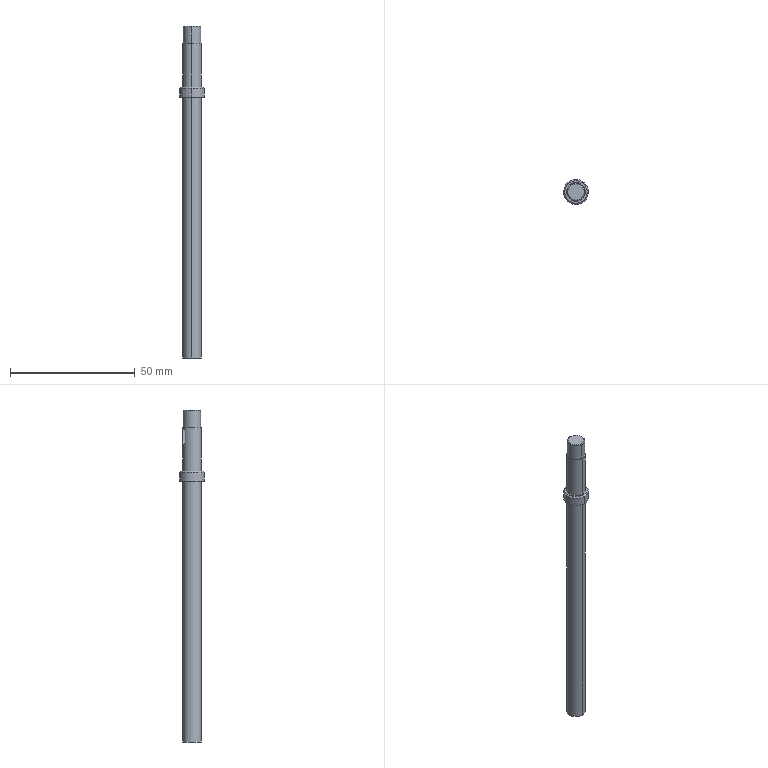Part | STEP file | 2026.6.15-Main Assembly图.sldasm-Part-112 | 1 solid | 22 faces | box 10 x 10 x 132.905 mm | volume 5947 mm3 | cylinder 10 | plane 8 | cone 4 | commonest cylinder face diameters 7.5 x4 2.5 x2 7 x2 10 x2
STEP:
#1=CARTESIAN_POINT('',(-1571.242,1419.764,3633.547));
#2=VERTEX_POINT('',#1);
#3=CARTESIAN_POINT('',(-1571.235,1428.764,3633.547));
#4=VERTEX_POINT('',#3);
#5=CARTESIAN_POINT('',(-1571.238,1424.264,3633.547));
#6=DIRECTION('',(0.,0.,1.));
#7=DIRECTION('',(-0.0007664,-1.,0.));
#8=AXIS2_PLACEMENT_3D('',#5,#6,#7);
#9=CIRCLE('',#8,4.5);
#10=EDGE_CURVE('',#2,#4,#9,.T.);
#11=ORIENTED_EDGE('',*,*,#10,.F.);
#12=CARTESIAN_POINT('',(-1571.242,1419.264,3633.047));
#13=VERTEX_POINT('',#12);
#14=CARTESIAN_POINT('',(-1571.242,1419.264,3633.047));
#15=DIRECTION('',(-0.000542,-0.7071,-0.7071));
#16=VECTOR('',#15,1000.);
#17=LINE('',#14,#16);
#18=EDGE_CURVE('',#2,#13,#17,.T.);
#19=ORIENTED_EDGE('',*,*,#18,.T.);
#20=CARTESIAN_POINT('',(-1571.044,1429.261,3633.047));
#21=VERTEX_POINT('',#20);
#22=CARTESIAN_POINT('',(-1571.238,1424.264,3633.047));
#23=DIRECTION('',(0.,0.,-1.));
#24=DIRECTION('',(-0.0007664,-1.,0.));
#25=AXIS2_PLACEMENT_3D('',#22,#23,#24);
#26=CIRCLE('',#25,5.);
#27=EDGE_CURVE('',#21,#13,#26,.T.);
#28=ORIENTED_EDGE('',*,*,#27,.F.);
#29=CARTESIAN_POINT('',(-1571.234,1429.264,3633.047));
#30=VERTEX_POINT('',#29);
#31=CARTESIAN_POINT('',(-1571.238,1424.264,3633.047));
#32=DIRECTION('',(0.,0.,-1.));
#33=DIRECTION('',(-0.0007664,-1.,0.));
#34=AXIS2_PLACEMENT_3D('',#31,#32,#33);
#35=CIRCLE('',#34,5.);
#36=EDGE_CURVE('',#30,#21,#35,.T.);
#37=ORIENTED_EDGE('',*,*,#36,.F.);
#38=CARTESIAN_POINT('',(-1571.234,1429.264,3633.047));
#39=DIRECTION('',(0.000542,0.7071,-0.7071));
#40=VECTOR('',#39,1000.);
#41=LINE('',#38,#40);
#42=EDGE_CURVE('',#4,#30,#41,.T.);
#43=ORIENTED_EDGE('',*,*,#42,.F.);
#44=EDGE_LOOP('',(#11,#19,#28,#37,#43));
#45=FACE_OUTER_BOUND('',#44,.T.);
#46=CARTESIAN_POINT('',(-1571.238,1424.264,3633.047));
#47=DIRECTION('',(0.,0.,-1.));
#48=DIRECTION('',(0.0007664,1.,0.));
#49=AXIS2_PLACEMENT_3D('',#46,#47,#48);
#50=CONICAL_SURFACE('',#49,5.,0.7854);
#51=ADVANCED_FACE('',(#45),#50,.T.);
#52=CARTESIAN_POINT('',(-1571.241,1421.014,3658.047));
#53=VERTEX_POINT('',#52);
#54=CARTESIAN_POINT('',(-1571.236,1427.514,3658.047));
#55=VERTEX_POINT('',#54);
#56=CARTESIAN_POINT('',(-1571.238,1424.264,3658.047));
#57=DIRECTION('',(0.,0.,1.));
#58=DIRECTION('',(-0.0007664,-1.,0.));
#59=AXIS2_PLACEMENT_3D('',#56,#57,#58);
#60=CIRCLE('',#59,3.25);
#61=EDGE_CURVE('',#53,#55,#60,.T.);
#62=ORIENTED_EDGE('',*,*,#61,.F.);
#63=CARTESIAN_POINT('',(-1571.241,1420.764,3657.797));
#64=VERTEX_POINT('',#63);
#65=CARTESIAN_POINT('',(-1571.241,1420.764,3657.797));
#66=DIRECTION('',(-0.000542,-0.7071,-0.7071));
#67=VECTOR('',#66,1000.);
#68=LINE('',#65,#67);
#69=EDGE_CURVE('',#53,#64,#68,.T.);
#70=ORIENTED_EDGE('',*,*,#69,.T.);
#71=CARTESIAN_POINT('',(-1571.102,1427.762,3657.797));
#72=VERTEX_POINT('',#71);
#73=CARTESIAN_POINT('',(-1571.238,1424.264,3657.797));
#74=DIRECTION('',(0.,0.,-1.));
#75=DIRECTION('',(-0.0007664,-1.,0.));
#76=AXIS2_PLACEMENT_3D('',#73,#74,#75);
#77=CIRCLE('',#76,3.5);
#78=EDGE_CURVE('',#72,#64,#77,.T.);
#79=ORIENTED_EDGE('',*,*,#78,.F.);
#80=CARTESIAN_POINT('',(-1571.236,1427.764,3657.797));
#81=VERTEX_POINT('',#80);
#82=CARTESIAN_POINT('',(-1571.238,1424.264,3657.797));
#83=DIRECTION('',(0.,0.,-1.));
#84=DIRECTION('',(-0.0007664,-1.,0.));
#85=AXIS2_PLACEMENT_3D('',#82,#83,#84);
#86=CIRCLE('',#85,3.5);
#87=EDGE_CURVE('',#81,#72,#86,.T.);
#88=ORIENTED_EDGE('',*,*,#87,.F.);
#89=CARTESIAN_POINT('',(-1571.236,1427.764,3657.797));
#90=DIRECTION('',(0.000542,0.7071,-0.7071));
#91=VECTOR('',#90,1000.);
#92=LINE('',#89,#91);
#93=EDGE_CURVE('',#55,#81,#92,.T.);
#94=ORIENTED_EDGE('',*,*,#93,.F.);
#95=EDGE_LOOP('',(#62,#70,#79,#88,#94));
#96=FACE_OUTER_BOUND('',#95,.T.);
#97=CARTESIAN_POINT('',(-1571.238,1424.264,3657.797));
#98=DIRECTION('',(0.,0.,-1.));
#99=DIRECTION('',(0.0007664,1.,0.));
#100=AXIS2_PLACEMENT_3D('',#97,#98,#99);
#101=CONICAL_SURFACE('',#100,3.5,0.7854);
#102=ADVANCED_FACE('',(#96),#101,.T.);
#103=ORIENTED_EDGE('',*,*,#27,.T.);
#104=CARTESIAN_POINT('',(-1571.433,1419.268,3633.047));
#105=VERTEX_POINT('',#104);
#106=CARTESIAN_POINT('',(-1571.238,1424.264,3633.047));
#107=DIRECTION('',(0.,0.,-1.));
#108=DIRECTION('',(-0.0007664,-1.,0.));
#109=AXIS2_PLACEMENT_3D('',#106,#107,#108);
#110=CIRCLE('',#109,5.);
#111=EDGE_CURVE('',#13,#105,#110,.T.);
#112=ORIENTED_EDGE('',*,*,#111,.T.);
#113=CARTESIAN_POINT('',(-1571.433,1419.268,3629.547));
#114=VERTEX_POINT('',#113);
#115=CARTESIAN_POINT('',(-1571.433,1419.268,3633.547));
#116=DIRECTION('',(0.,0.,-1.));
#117=VECTOR('',#116,1000.);
#118=LINE('',#115,#117);
#119=EDGE_CURVE('',#105,#114,#118,.T.);
#120=ORIENTED_EDGE('',*,*,#119,.T.);
#121=CARTESIAN_POINT('',(-1571.044,1429.261,3629.547));
#122=VERTEX_POINT('',#121);
#123=CARTESIAN_POINT('',(-1571.238,1424.264,3629.547));
#124=DIRECTION('',(0.,0.,1.));
#125=DIRECTION('',(0.03892,0.9992,0.));
#126=AXIS2_PLACEMENT_3D('',#123,#124,#125);
#127=CIRCLE('',#126,5.);
#128=EDGE_CURVE('',#114,#122,#127,.T.);
#129=ORIENTED_EDGE('',*,*,#128,.T.);
#130=CARTESIAN_POINT('',(-1571.044,1429.261,3633.547));
#131=DIRECTION('',(0.,0.,-1.));
#132=VECTOR('',#131,1000.);
#133=LINE('',#130,#132);
#134=EDGE_CURVE('',#21,#122,#133,.T.);
#135=ORIENTED_EDGE('',*,*,#134,.F.);
#136=EDGE_LOOP('',(#103,#112,#120,#129,#135));
#137=FACE_OUTER_BOUND('',#136,.T.);
#138=CARTESIAN_POINT('',(-1571.238,1424.264,3633.547));
#139=DIRECTION('',(0.,0.,-1.));
#140=DIRECTION('',(0.03892,0.9992,0.));
#141=AXIS2_PLACEMENT_3D('',#138,#139,#140);
#142=CYLINDRICAL_SURFACE('',#141,5.);
#143=ADVANCED_FACE('',(#137),#142,.T.);
#144=CARTESIAN_POINT('',(-1571.092,1428.011,3651.047));
#145=VERTEX_POINT('',#144);
#146=CARTESIAN_POINT('',(-1571.384,1420.517,3651.047));
#147=VERTEX_POINT('',#146);
#148=CARTESIAN_POINT('',(-1571.238,1424.264,3651.047));
#149=DIRECTION('',(0.,0.,-1.));
#150=DIRECTION('',(0.03892,0.9992,0.));
#151=AXIS2_PLACEMENT_3D('',#148,#149,#150);
#152=CIRCLE('',#151,3.75);
#153=EDGE_CURVE('',#145,#147,#152,.T.);
#154=ORIENTED_EDGE('',*,*,#153,.T.);
#155=CARTESIAN_POINT('',(-1571.384,1420.517,3633.547));
#156=VERTEX_POINT('',#155);
#157=CARTESIAN_POINT('',(-1571.384,1420.517,3651.047));
#158=DIRECTION('',(0.,0.,-1.));
#159=VECTOR('',#158,1000.);
#160=LINE('',#157,#159);
#161=EDGE_CURVE('',#147,#156,#160,.T.);
#162=ORIENTED_EDGE('',*,*,#161,.T.);
#163=CARTESIAN_POINT('',(-1571.092,1428.011,3633.547));
#164=VERTEX_POINT('',#163);
#165=CARTESIAN_POINT('',(-1571.238,1424.264,3633.547));
#166=DIRECTION('',(0.,0.,1.));
#167=DIRECTION('',(0.03892,0.9992,0.));
#168=AXIS2_PLACEMENT_3D('',#165,#166,#167);
#169=CIRCLE('',#168,3.75);
#170=EDGE_CURVE('',#156,#164,#169,.T.);
#171=ORIENTED_EDGE('',*,*,#170,.T.);
#172=CARTESIAN_POINT('',(-1571.092,1428.011,3651.047));
#173=DIRECTION('',(0.,0.,-1.));
#174=VECTOR('',#173,1000.);
#175=LINE('',#172,#174);
#176=EDGE_CURVE('',#145,#164,#175,.T.);
#177=ORIENTED_EDGE('',*,*,#176,.F.);
#178=EDGE_LOOP('',(#154,#162,#171,#177));
#179=FACE_OUTER_BOUND('',#178,.T.);
#180=CARTESIAN_POINT('',(-1571.238,1424.264,3651.047));
#181=DIRECTION('',(0.,0.,-1.));
#182=DIRECTION('',(0.03892,0.9992,0.));
#183=AXIS2_PLACEMENT_3D('',#180,#181,#182);
#184=CYLINDRICAL_SURFACE('',#183,3.75);
#185=ADVANCED_FACE('',(#179),#184,.T.);
#186=ORIENTED_EDGE('',*,*,#78,.T.);
#187=CARTESIAN_POINT('',(-1571.374,1420.767,3657.797));
#188=VERTEX_POINT('',#187);
#189=CARTESIAN_POINT('',(-1571.238,1424.264,3657.797));
#190=DIRECTION('',(0.,0.,-1.));
#191=DIRECTION('',(-0.0007664,-1.,0.));
#192=AXIS2_PLACEMENT_3D('',#189,#190,#191);
#193=CIRCLE('',#192,3.5);
#194=EDGE_CURVE('',#64,#188,#193,.T.);
#195=ORIENTED_EDGE('',*,*,#194,.T.);
#196=CARTESIAN_POINT('',(-1571.374,1420.767,3651.047));
#197=VERTEX_POINT('',#196);
#198=CARTESIAN_POINT('',(-1571.374,1420.767,3658.047));
#199=DIRECTION('',(0.,0.,-1.));
#200=VECTOR('',#199,1000.);
#201=LINE('',#198,#200);
#202=EDGE_CURVE('',#188,#197,#201,.T.);
#203=ORIENTED_EDGE('',*,*,#202,.T.);
#204=CARTESIAN_POINT('',(-1571.102,1427.762,3651.047));
#205=VERTEX_POINT('',#204);
#206=CARTESIAN_POINT('',(-1571.238,1424.264,3651.047));
#207=DIRECTION('',(0.,0.,1.));
#208=DIRECTION('',(0.03892,0.9992,0.));
#209=AXIS2_PLACEMENT_3D('',#206,#207,#208);
#210=CIRCLE('',#209,3.5);
#211=EDGE_CURVE('',#197,#205,#210,.T.);
#212=ORIENTED_EDGE('',*,*,#211,.T.);
#213=CARTESIAN_POINT('',(-1571.102,1427.762,3658.047));
#214=DIRECTION('',(0.,0.,-1.));
#215=VECTOR('',#214,1000.);
#216=LINE('',#213,#215);
#217=EDGE_CURVE('',#72,#205,#216,.T.);
#218=ORIENTED_EDGE('',*,*,#217,.F.);
#219=EDGE_LOOP('',(#186,#195,#203,#212,#218));
#220=FACE_OUTER_BOUND('',#219,.T.);
#221=CARTESIAN_POINT('',(-1571.238,1424.264,3658.047));
#222=DIRECTION('',(0.,0.,-1.));
#223=DIRECTION('',(0.03892,0.9992,0.));
#224=AXIS2_PLACEMENT_3D('',#221,#222,#223);
#225=CYLINDRICAL_SURFACE('',#224,3.5);
#226=ADVANCED_FACE('',(#220),#225,.T.);
#227=CARTESIAN_POINT('',(-1571.092,1428.011,3629.547));
#228=VERTEX_POINT('',#227);
#229=CARTESIAN_POINT('',(-1571.384,1420.517,3629.547));
#230=VERTEX_POINT('',#229);
#231=CARTESIAN_POINT('',(-1571.238,1424.264,3629.547));
#232=DIRECTION('',(0.,0.,-1.));
#233=DIRECTION('',(0.03892,0.9992,0.));
#234=AXIS2_PLACEMENT_3D('',#231,#232,#233);
#235=CIRCLE('',#234,3.75);
#236=EDGE_CURVE('',#228,#230,#235,.T.);
#237=ORIENTED_EDGE('',*,*,#236,.T.);
#238=CARTESIAN_POINT('',(-1571.384,1420.517,3525.142));
#239=VERTEX_POINT('',#238);
#240=CARTESIAN_POINT('',(-1571.384,1420.517,3629.547));
#241=DIRECTION('',(0.,0.,-1.));
#242=VECTOR('',#241,1000.);
#243=LINE('',#240,#242);
#244=EDGE_CURVE('',#230,#239,#243,.T.);
#245=ORIENTED_EDGE('',*,*,#244,.T.);
#246=CARTESIAN_POINT('',(-1571.092,1428.011,3525.142));
#247=VERTEX_POINT('',#246);
#248=CARTESIAN_POINT('',(-1571.238,1424.264,3525.142));
#249=DIRECTION('',(0.,0.,-1.));
#250=DIRECTION('',(1.,0.,0.));
#251=AXIS2_PLACEMENT_3D('',#248,#249,#250);
#252=CIRCLE('',#251,3.75);
#253=EDGE_CURVE('',#247,#239,#252,.T.);
#254=ORIENTED_EDGE('',*,*,#253,.F.);
#255=CARTESIAN_POINT('',(-1571.092,1428.011,3629.547));
#256=DIRECTION('',(0.,0.,-1.));
#257=VECTOR('',#256,1000.);
#258=LINE('',#255,#257);
#259=EDGE_CURVE('',#228,#247,#258,.T.);
#260=ORIENTED_EDGE('',*,*,#259,.F.);
#261=EDGE_LOOP('',(#237,#245,#254,#260));
#262=FACE_OUTER_BOUND('',#261,.T.);
#263=CARTESIAN_POINT('',(-1571.238,1424.264,3629.547));
#264=DIRECTION('',(0.,0.,-1.));
#265=DIRECTION('',(0.03892,0.9992,0.));
#266=AXIS2_PLACEMENT_3D('',#263,#264,#265);
#267=CYLINDRICAL_SURFACE('',#266,3.75);
#268=ADVANCED_FACE('',(#262),#267,.T.);
#269=ORIENTED_EDGE('',*,*,#244,.F.);
#270=CARTESIAN_POINT('',(-1571.238,1424.264,3629.547));
#271=DIRECTION('',(0.,0.,-1.));
#272=DIRECTION('',(0.03892,0.9992,0.));
#273=AXIS2_PLACEMENT_3D('',#270,#271,#272);
#274=CIRCLE('',#273,3.75);
#275=EDGE_CURVE('',#230,#228,#274,.T.);
#276=ORIENTED_EDGE('',*,*,#275,.T.);
#277=ORIENTED_EDGE('',*,*,#259,.T.);
#278=CARTESIAN_POINT('',(-1571.238,1424.264,3525.142));
#279=DIRECTION('',(0.,0.,-1.));
#280=DIRECTION('',(1.,0.,0.));
#281=AXIS2_PLACEMENT_3D('',#278,#279,#280);
#282=CIRCLE('',#281,3.75);
#283=EDGE_CURVE('',#239,#247,#282,.T.);
#284=ORIENTED_EDGE('',*,*,#283,.F.);
#285=EDGE_LOOP('',(#269,#276,#277,#284));
#286=FACE_OUTER_BOUND('',#285,.T.);
#287=CARTESIAN_POINT('',(-1571.238,1424.264,3629.547));
#288=DIRECTION('',(0.,0.,-1.));
#289=DIRECTION('',(0.03892,0.9992,0.));
#290=AXIS2_PLACEMENT_3D('',#287,#288,#289);
#291=CYLINDRICAL_SURFACE('',#290,3.75);
#292=ADVANCED_FACE('',(#286),#291,.T.);
#293=CARTESIAN_POINT('',(-1571.238,1424.264,3658.047));
#294=DIRECTION('',(0.,0.,1.));
#295=DIRECTION('',(-0.0007664,-1.,0.));
#296=AXIS2_PLACEMENT_3D('',#293,#294,#295);
#297=CIRCLE('',#296,3.25);
#298=EDGE_CURVE('',#55,#53,#297,.T.);
#299=ORIENTED_EDGE('',*,*,#298,.T.);
#300=ORIENTED_EDGE('',*,*,#61,.T.);
#301=EDGE_LOOP('',(#299,#300));
#302=FACE_OUTER_BOUND('',#301,.T.);
#303=CARTESIAN_POINT('',(-1571.238,1424.264,3658.047));
#304=DIRECTION('',(0.,0.,1.));
#305=DIRECTION('',(-0.0007664,-1.,0.));
#306=AXIS2_PLACEMENT_3D('',#303,#304,#305);
#307=PLANE('',#306);
#308=ADVANCED_FACE('',(#302),#307,.T.);
#309=ORIENTED_EDGE('',*,*,#202,.F.);
#310=CARTESIAN_POINT('',(-1571.238,1424.264,3657.797));
#311=DIRECTION('',(0.,0.,-1.));
#312=DIRECTION('',(-0.0007664,-1.,0.));
#313=AXIS2_PLACEMENT_3D('',#310,#311,#312);
#314=CIRCLE('',#313,3.5);
#315=EDGE_CURVE('',#188,#81,#314,.T.);
#316=ORIENTED_EDGE('',*,*,#315,.T.);
#317=ORIENTED_EDGE('',*,*,#87,.T.);
#318=ORIENTED_EDGE('',*,*,#217,.T.);
#319=CARTESIAN_POINT('',(-1571.238,1424.264,3651.047));
#320=DIRECTION('',(0.,0.,1.));
#321=DIRECTION('',(0.03892,0.9992,0.));
#322=AXIS2_PLACEMENT_3D('',#319,#320,#321);
#323=CIRCLE('',#322,3.5);
#324=EDGE_CURVE('',#205,#197,#323,.T.);
#325=ORIENTED_EDGE('',*,*,#324,.T.);
#326=EDGE_LOOP('',(#309,#316,#317,#318,#325));
#327=FACE_OUTER_BOUND('',#326,.T.);
#328=CARTESIAN_POINT('',(-1571.238,1424.264,3658.047));
#329=DIRECTION('',(0.,0.,-1.));
#330=DIRECTION('',(0.03892,0.9992,0.));
#331=AXIS2_PLACEMENT_3D('',#328,#329,#330);
#332=CYLINDRICAL_SURFACE('',#331,3.5);
#333=ADVANCED_FACE('',(#327),#332,.T.);
#334=ORIENTED_EDGE('',*,*,#324,.F.);
#335=ORIENTED_EDGE('',*,*,#211,.F.);
#336=EDGE_LOOP('',(#334,#335));
#337=FACE_BOUND('',#336,.T.);
#338=ORIENTED_EDGE('',*,*,#153,.F.);
#339=CARTESIAN_POINT('',(-1571.238,1424.264,3651.047));
#340=DIRECTION('',(0.,0.,-1.));
#341=DIRECTION('',(0.03892,0.9992,0.));
#342=AXIS2_PLACEMENT_3D('',#339,#340,#341);
#343=CIRCLE('',#342,3.75);
#344=EDGE_CURVE('',#147,#145,#343,.T.);
#345=ORIENTED_EDGE('',*,*,#344,.F.);
#346=EDGE_LOOP('',(#338,#345));
#347=FACE_OUTER_BOUND('',#346,.T.);
#348=CARTESIAN_POINT('',(-1571.238,1424.264,3651.047));
#349=DIRECTION('',(0.,0.,1.));
#350=DIRECTION('',(-0.0007664,-1.,0.));
#351=AXIS2_PLACEMENT_3D('',#348,#349,#350);
#352=PLANE('',#351);
#353=ADVANCED_FACE('',(#337,#347),#352,.T.);
#354=ORIENTED_EDGE('',*,*,#161,.F.);
#355=ORIENTED_EDGE('',*,*,#344,.T.);
#356=ORIENTED_EDGE('',*,*,#176,.T.);
#357=CARTESIAN_POINT('',(-1571.238,1424.264,3633.547));
#358=DIRECTION('',(0.,0.,1.));
#359=DIRECTION('',(0.03892,0.9992,0.));
#360=AXIS2_PLACEMENT_3D('',#357,#358,#359);
#361=CIRCLE('',#360,3.75);
#362=EDGE_CURVE('',#164,#156,#361,.T.);
#363=ORIENTED_EDGE('',*,*,#362,.T.);
#364=EDGE_LOOP('',(#354,#355,#356,#363));
#365=FACE_OUTER_BOUND('',#364,.T.);
#366=CARTESIAN_POINT('',(-1571.607,1427.996,3645.547));
#367=VERTEX_POINT('',#366);
#368=CARTESIAN_POINT('',(-1573.871,1426.935,3645.547));
#369=VERTEX_POINT('',#368);
#370=CARTESIAN_POINT('',(-1571.607,1427.996,3645.547));
#371=CARTESIAN_POINT('',(-1571.607,1427.996,3645.38));
#372=CARTESIAN_POINT('',(-1571.642,1427.993,3645.217));
#373=CARTESIAN_POINT('',(-1571.773,1427.977,3644.915));
#374=CARTESIAN_POINT('',(-1571.869,1427.963,3644.777));
#375=CARTESIAN_POINT('',(-1572.1,1427.916,3644.549));
#376=CARTESIAN_POINT('',(-1572.237,1427.882,3644.456));
#377=CARTESIAN_POINT('',(-1572.525,1427.79,3644.331));
#378=CARTESIAN_POINT('',(-1572.68,1427.73,3644.297));
#379=CARTESIAN_POINT('',(-1572.903,1427.626,3644.297));
#380=CARTESIAN_POINT('',(-1572.977,1427.588,3644.305));
#381=CARTESIAN_POINT('',(-1573.119,1427.51,3644.337));
#382=CARTESIAN_POINT('',(-1573.186,1427.47,3644.361));
#383=CARTESIAN_POINT('',(-1573.38,1427.346,3644.456));
#384=CARTESIAN_POINT('',(-1573.493,1427.263,3644.548));
#385=CARTESIAN_POINT('',(-1573.631,1427.152,3644.72));
#386=CARTESIAN_POINT('',(-1573.672,1427.118,3644.783));
#387=CARTESIAN_POINT('',(-1573.743,1427.056,3644.918));
#388=CARTESIAN_POINT('',(-1573.773,1427.028,3644.991));
#389=CARTESIAN_POINT('',(-1573.845,1426.961,3645.216));
#390=CARTESIAN_POINT('',(-1573.871,1426.935,3645.38));
#391=CARTESIAN_POINT('',(-1573.871,1426.935,3645.547));
#392=B_SPLINE_CURVE_WITH_KNOTS('',3,(#370,#371,#372,#373,#374,#375,#376,#377,#378,#379,#380,#381,#382,#383,#384,#385,#386,#387,#388,#389,#390,#391),.UNSPECIFIED.,.F.,.F.,(4,2,2,2,2,2,2,2,2,2,4),(0.,0.0004919,0.0009837,0.001476,0.001967,0.002213,0.002459,0.002951,0.003197,0.003443,0.003935),.UNSPECIFIED.);
#393=EDGE_CURVE('',#367,#369,#392,.T.);
#394=ORIENTED_EDGE('',*,*,#393,.F.);
#395=CARTESIAN_POINT('',(-1571.607,1427.996,3649.547));
#396=VERTEX_POINT('',#395);
#397=CARTESIAN_POINT('',(-1571.607,1427.996,3651.047));
#398=DIRECTION('',(0.,0.,1.));
#399=VECTOR('',#398,1000.);
#400=LINE('',#397,#399);
#401=EDGE_CURVE('',#367,#396,#400,.T.);
#402=ORIENTED_EDGE('',*,*,#401,.T.);
#403=CARTESIAN_POINT('',(-1573.871,1426.935,3649.547));
#404=VERTEX_POINT('',#403);
#405=CARTESIAN_POINT('',(-1573.871,1426.935,3649.547));
#406=CARTESIAN_POINT('',(-1573.871,1426.935,3649.713));
#407=CARTESIAN_POINT('',(-1573.846,1426.96,3649.876));
#408=CARTESIAN_POINT('',(-1573.749,1427.05,3650.178));
#409=CARTESIAN_POINT('',(-1573.677,1427.115,3650.316));
#410=CARTESIAN_POINT('',(-1573.494,1427.263,3650.545));
#411=CARTESIAN_POINT('',(-1573.38,1427.346,3650.638));
#412=CARTESIAN_POINT('',(-1573.125,1427.509,3650.763));
#413=CARTESIAN_POINT('',(-1572.98,1427.589,3650.797));
#414=CARTESIAN_POINT('',(-1572.757,1427.694,3650.797));
#415=CARTESIAN_POINT('',(-1572.68,1427.727,3650.789));
#416=CARTESIAN_POINT('',(-1572.53,1427.786,3650.757));
#417=CARTESIAN_POINT('',(-1572.456,1427.812,3650.733));
#418=CARTESIAN_POINT('',(-1572.237,1427.882,3650.638));
#419=CARTESIAN_POINT('',(-1572.101,1427.916,3650.546));
#420=CARTESIAN_POINT('',(-1571.927,1427.951,3650.373));
#421=CARTESIAN_POINT('',(-1571.874,1427.96,3650.311));
#422=CARTESIAN_POINT('',(-1571.781,1427.975,3650.176));
#423=CARTESIAN_POINT('',(-1571.741,1427.981,3650.103));
#424=CARTESIAN_POINT('',(-1571.643,1427.993,3649.878));
#425=CARTESIAN_POINT('',(-1571.607,1427.996,3649.713));
#426=CARTESIAN_POINT('',(-1571.607,1427.996,3649.547));
#427=B_SPLINE_CURVE_WITH_KNOTS('',3,(#405,#406,#407,#408,#409,#410,#411,#412,#413,#414,#415,#416,#417,#418,#419,#420,#421,#422,#423,#424,#425,#426),.UNSPECIFIED.,.F.,.F.,(4,2,2,2,2,2,2,2,2,2,4),(0.,0.0004919,0.0009837,0.001476,0.001967,0.002213,0.002459,0.002951,0.003197,0.003443,0.003935),.UNSPECIFIED.);
#428=EDGE_CURVE('',#404,#396,#427,.T.);
#429=ORIENTED_EDGE('',*,*,#428,.F.);
#430=CARTESIAN_POINT('',(-1573.871,1426.935,3651.047));
#431=DIRECTION('',(0.,0.,-1.));
#432=VECTOR('',#431,1000.);
#433=LINE('',#430,#432);
#434=EDGE_CURVE('',#404,#369,#433,.T.);
#435=ORIENTED_EDGE('',*,*,#434,.T.);
#436=EDGE_LOOP('',(#394,#402,#429,#435));
#437=FACE_BOUND('',#436,.T.);
#438=CARTESIAN_POINT('',(-1571.238,1424.264,3651.047));
#439=DIRECTION('',(0.,0.,-1.));
#440=DIRECTION('',(0.03892,0.9992,0.));
#441=AXIS2_PLACEMENT_3D('',#438,#439,#440);
#442=CYLINDRICAL_SURFACE('',#441,3.75);
#443=ADVANCED_FACE('',(#365,#437),#442,.T.);
#444=ORIENTED_EDGE('',*,*,#236,.F.);
#445=ORIENTED_EDGE('',*,*,#275,.F.);
#446=EDGE_LOOP('',(#444,#445));
#447=FACE_BOUND('',#446,.T.);
#448=CARTESIAN_POINT('',(-1571.238,1424.264,3629.547));
#449=DIRECTION('',(0.,0.,1.));
#450=DIRECTION('',(0.03892,0.9992,0.));
#451=AXIS2_PLACEMENT_3D('',#448,#449,#450);
#452=CIRCLE('',#451,5.);
#453=EDGE_CURVE('',#122,#114,#452,.T.);
#454=ORIENTED_EDGE('',*,*,#453,.F.);
#455=ORIENTED_EDGE('',*,*,#128,.F.);
#456=EDGE_LOOP('',(#454,#455));
#457=FACE_OUTER_BOUND('',#456,.T.);
#458=CARTESIAN_POINT('',(-1571.238,1424.264,3629.547));
#459=DIRECTION('',(0.,0.,-1.));
#460=DIRECTION('',(0.0007664,1.,0.));
#461=AXIS2_PLACEMENT_3D('',#458,#459,#460);
#462=PLANE('',#461);
#463=ADVANCED_FACE('',(#447,#457),#462,.T.);
#464=CARTESIAN_POINT('',(-1571.238,1424.264,3633.547));
#465=DIRECTION('',(0.,0.,1.));
#466=DIRECTION('',(-0.0007664,-1.,0.));
#467=AXIS2_PLACEMENT_3D('',#464,#465,#466);
#468=CIRCLE('',#467,4.5);
#469=EDGE_CURVE('',#4,#2,#468,.T.);
#470=ORIENTED_EDGE('',*,*,#469,.T.);
#471=ORIENTED_EDGE('',*,*,#10,.T.);
#472=EDGE_LOOP('',(#470,#471));
#473=FACE_OUTER_BOUND('',#472,.T.);
#474=ORIENTED_EDGE('',*,*,#362,.F.);
#475=ORIENTED_EDGE('',*,*,#170,.F.);
#476=EDGE_LOOP('',(#474,#475));
#477=FACE_BOUND('',#476,.T.);
#478=CARTESIAN_POINT('',(-1571.238,1424.264,3633.547));
#479=DIRECTION('',(0.,0.,1.));
#480=DIRECTION('',(-0.0007664,-1.,0.));
#481=AXIS2_PLACEMENT_3D('',#478,#479,#480);
#482=PLANE('',#481);
#483=ADVANCED_FACE('',(#473,#477),#482,.T.);
#484=ORIENTED_EDGE('',*,*,#119,.F.);
#485=CARTESIAN_POINT('',(-1571.238,1424.264,3633.047));
#486=DIRECTION('',(0.,0.,-1.));
#487=DIRECTION('',(-0.0007664,-1.,0.));
#488=AXIS2_PLACEMENT_3D('',#485,#486,#487);
#489=CIRCLE('',#488,5.);
#490=EDGE_CURVE('',#105,#30,#489,.T.);
#491=ORIENTED_EDGE('',*,*,#490,.T.);
#492=ORIENTED_EDGE('',*,*,#36,.T.);
#493=ORIENTED_EDGE('',*,*,#134,.T.);
#494=ORIENTED_EDGE('',*,*,#453,.T.);
#495=EDGE_LOOP('',(#484,#491,#492,#493,#494));
#496=FACE_OUTER_BOUND('',#495,.T.);
#497=CARTESIAN_POINT('',(-1571.238,1424.264,3633.547));
#498=DIRECTION('',(0.,0.,-1.));
#499=DIRECTION('',(0.03892,0.9992,0.));
#500=AXIS2_PLACEMENT_3D('',#497,#498,#499);
#501=CYLINDRICAL_SURFACE('',#500,5.);
#502=ADVANCED_FACE('',(#496),#501,.T.);
#503=ORIENTED_EDGE('',*,*,#69,.F.);
#504=ORIENTED_EDGE('',*,*,#298,.F.);
#505=ORIENTED_EDGE('',*,*,#93,.T.);
#506=ORIENTED_EDGE('',*,*,#315,.F.);
#507=ORIENTED_EDGE('',*,*,#194,.F.);
#508=EDGE_LOOP('',(#503,#504,#505,#506,#507));
#509=FACE_OUTER_BOUND('',#508,.T.);
#510=CARTESIAN_POINT('',(-1571.238,1424.264,3657.797));
#511=DIRECTION('',(0.,0.,-1.));
#512=DIRECTION('',(0.0007664,1.,0.));
#513=AXIS2_PLACEMENT_3D('',#510,#511,#512);
#514=CONICAL_SURFACE('',#513,3.5,0.7854);
#515=ADVANCED_FACE('',(#509),#514,.T.);
#516=ORIENTED_EDGE('',*,*,#18,.F.);
#517=ORIENTED_EDGE('',*,*,#469,.F.);
#518=ORIENTED_EDGE('',*,*,#42,.T.);
#519=ORIENTED_EDGE('',*,*,#490,.F.);
#520=ORIENTED_EDGE('',*,*,#111,.F.);
#521=EDGE_LOOP('',(#516,#517,#518,#519,#520));
#522=FACE_OUTER_BOUND('',#521,.T.);
#523=CARTESIAN_POINT('',(-1571.238,1424.264,3633.047));
#524=DIRECTION('',(0.,0.,-1.));
#525=DIRECTION('',(0.0007664,1.,0.));
#526=AXIS2_PLACEMENT_3D('',#523,#524,#525);
#527=CONICAL_SURFACE('',#526,5.,0.7854);
#528=ADVANCED_FACE('',(#522),#527,.T.);
#529=CARTESIAN_POINT('',(-1573.431,1425.997,3649.547));
#530=VERTEX_POINT('',#529);
#531=CARTESIAN_POINT('',(-1573.431,1425.997,3649.547));
#532=DIRECTION('',(0.4244,-0.9055,0.));
#533=VECTOR('',#532,1000.);
#534=LINE('',#531,#533);
#535=EDGE_CURVE('',#404,#530,#534,.T.);
#536=ORIENTED_EDGE('',*,*,#535,.T.);
#537=CARTESIAN_POINT('',(-1573.431,1425.997,3645.547));
#538=VERTEX_POINT('',#537);
#539=CARTESIAN_POINT('',(-1573.431,1425.997,3650.797));
#540=DIRECTION('',(0.,0.,-1.));
#541=VECTOR('',#540,1000.);
#542=LINE('',#539,#541);
#543=EDGE_CURVE('',#530,#538,#542,.T.);
#544=ORIENTED_EDGE('',*,*,#543,.T.);
#545=CARTESIAN_POINT('',(-1573.431,1425.997,3645.547));
#546=DIRECTION('',(-0.4244,0.9055,0.));
#547=VECTOR('',#546,1000.);
#548=LINE('',#545,#547);
#549=EDGE_CURVE('',#538,#369,#548,.T.);
#550=ORIENTED_EDGE('',*,*,#549,.T.);
#551=ORIENTED_EDGE('',*,*,#434,.F.);
#552=EDGE_LOOP('',(#536,#544,#550,#551));
#553=FACE_OUTER_BOUND('',#552,.T.);
#554=CARTESIAN_POINT('',(-1573.431,1425.997,3650.797));
#555=DIRECTION('',(-0.9055,-0.4244,0.));
#556=DIRECTION('',(0.,0.,-1.));
#557=AXIS2_PLACEMENT_3D('',#554,#555,#556);
#558=PLANE('',#557);
#559=ADVANCED_FACE('',(#553),#558,.F.);
#560=CARTESIAN_POINT('',(-1571.167,1427.059,3645.547));
#561=VERTEX_POINT('',#560);
#562=CARTESIAN_POINT('',(-1571.167,1427.059,3645.547));
#563=DIRECTION('',(0.4244,-0.9055,0.));
#564=VECTOR('',#563,1000.);
#565=LINE('',#562,#564);
#566=EDGE_CURVE('',#367,#561,#565,.T.);
#567=ORIENTED_EDGE('',*,*,#566,.T.);
#568=CARTESIAN_POINT('',(-1571.167,1427.059,3649.547));
#569=VERTEX_POINT('',#568);
#570=CARTESIAN_POINT('',(-1571.167,1427.059,3650.797));
#571=DIRECTION('',(0.,0.,-1.));
#572=VECTOR('',#571,1000.);
#573=LINE('',#570,#572);
#574=EDGE_CURVE('',#569,#561,#573,.T.);
#575=ORIENTED_EDGE('',*,*,#574,.F.);
#576=CARTESIAN_POINT('',(-1571.167,1427.059,3649.547));
#577=DIRECTION('',(-0.4244,0.9055,0.));
#578=VECTOR('',#577,1000.);
#579=LINE('',#576,#578);
#580=EDGE_CURVE('',#569,#396,#579,.T.);
#581=ORIENTED_EDGE('',*,*,#580,.T.);
#582=ORIENTED_EDGE('',*,*,#401,.F.);
#583=EDGE_LOOP('',(#567,#575,#581,#582));
#584=FACE_OUTER_BOUND('',#583,.T.);
#585=CARTESIAN_POINT('',(-1571.167,1427.059,3650.797));
#586=DIRECTION('',(-0.9055,-0.4244,0.));
#587=DIRECTION('',(0.,0.,-1.));
#588=AXIS2_PLACEMENT_3D('',#585,#586,#587);
#589=PLANE('',#588);
#590=ADVANCED_FACE('',(#584),#589,.T.);
#591=ORIENTED_EDGE('',*,*,#574,.T.);
#592=CARTESIAN_POINT('',(-1572.299,1426.528,3645.547));
#593=DIRECTION('',(-0.4244,0.9055,0.));
#594=DIRECTION('',(0.9052,0.4243,0.02473));
#595=AXIS2_PLACEMENT_3D('',#592,#593,#594);
#596=CIRCLE('',#595,1.25);
#597=EDGE_CURVE('',#561,#538,#596,.T.);
#598=ORIENTED_EDGE('',*,*,#597,.T.);
#599=ORIENTED_EDGE('',*,*,#543,.F.);
#600=CARTESIAN_POINT('',(-1572.299,1426.528,3649.547));
#601=DIRECTION('',(-0.4244,0.9055,0.));
#602=DIRECTION('',(0.9052,0.4243,0.02473));
#603=AXIS2_PLACEMENT_3D('',#600,#601,#602);
#604=CIRCLE('',#603,1.25);
#605=EDGE_CURVE('',#530,#569,#604,.T.);
#606=ORIENTED_EDGE('',*,*,#605,.T.);
#607=EDGE_LOOP('',(#591,#598,#599,#606));
#608=FACE_OUTER_BOUND('',#607,.T.);
#609=CARTESIAN_POINT('',(-1573.431,1425.997,3650.797));
#610=DIRECTION('',(0.4244,-0.9055,0.));
#611=DIRECTION('',(0.9052,0.4243,0.02473));
#612=AXIS2_PLACEMENT_3D('',#609,#610,#611);
#613=PLANE('',#612);
#614=ADVANCED_FACE('',(#608),#613,.F.);
#615=ORIENTED_EDGE('',*,*,#393,.T.);
#616=ORIENTED_EDGE('',*,*,#549,.F.);
#617=ORIENTED_EDGE('',*,*,#597,.F.);
#618=ORIENTED_EDGE('',*,*,#566,.F.);
#619=EDGE_LOOP('',(#615,#616,#617,#618));
#620=FACE_OUTER_BOUND('',#619,.T.);
#621=CARTESIAN_POINT('',(-1572.299,1426.528,3645.547));
#622=DIRECTION('',(0.4244,-0.9055,0.));
#623=DIRECTION('',(0.9052,0.4243,0.02473));
#624=AXIS2_PLACEMENT_3D('',#621,#622,#623);
#625=CYLINDRICAL_SURFACE('',#624,1.25);
#626=ADVANCED_FACE('',(#620),#625,.F.);
#627=ORIENTED_EDGE('',*,*,#428,.T.);
#628=ORIENTED_EDGE('',*,*,#580,.F.);
#629=ORIENTED_EDGE('',*,*,#605,.F.);
#630=ORIENTED_EDGE('',*,*,#535,.F.);
#631=EDGE_LOOP('',(#627,#628,#629,#630));
#632=FACE_OUTER_BOUND('',#631,.T.);
#633=CARTESIAN_POINT('',(-1572.299,1426.528,3649.547));
#634=DIRECTION('',(-0.4244,0.9055,0.));
#635=DIRECTION('',(-0.9052,-0.4243,-0.02473));
#636=AXIS2_PLACEMENT_3D('',#633,#634,#635);
#637=CYLINDRICAL_SURFACE('',#636,1.25);
#638=ADVANCED_FACE('',(#632),#637,.F.);
#639=ORIENTED_EDGE('',*,*,#253,.T.);
#640=ORIENTED_EDGE('',*,*,#283,.T.);
#641=EDGE_LOOP('',(#639,#640));
#642=FACE_OUTER_BOUND('',#641,.T.);
#643=CARTESIAN_POINT('',(-1556.42,1410.832,3525.142));
#644=DIRECTION('',(0.,0.,1.));
#645=DIRECTION('',(1.,0.,0.));
#646=AXIS2_PLACEMENT_3D('',#643,#644,#645);
#647=PLANE('',#646);
#648=ADVANCED_FACE('',(#642),#647,.F.);
#649=CLOSED_SHELL('',(#51,#102,#143,#185,#226,#268,#292,#308,#333,#353,#443,#463,#483,#502,#515,#528,#559,#590,#614,#626,#638,#648));
#650=MANIFOLD_SOLID_BREP('',#649);
#651=CARTESIAN_POINT('',(0.,0.,0.));
#652=DIRECTION('',(0.,0.,1.));
#653=DIRECTION('',(1.,0.,0.));
#654=AXIS2_PLACEMENT_3D('',#651,#652,#653);
#655=(LENGTH_UNIT()NAMED_UNIT(*)SI_UNIT(.MILLI.,.METRE.));
#656=UNCERTAINTY_MEASURE_WITH_UNIT(LENGTH_MEASURE(0.00001),#655,'','');
#657=(NAMED_UNIT(*)PLANE_ANGLE_UNIT()SI_UNIT($,.RADIAN.));
#658=(NAMED_UNIT(*)SI_UNIT($,.STERADIAN.)SOLID_ANGLE_UNIT());
#659=(GEOMETRIC_REPRESENTATION_CONTEXT(3)GLOBAL_UNCERTAINTY_ASSIGNED_CONTEXT((#656))GLOBAL_UNIT_ASSIGNED_CONTEXT((#655,#657,#658))REPRESENTATION_CONTEXT('',''));
#660=ADVANCED_BREP_SHAPE_REPRESENTATION('',(#650,#654),#659);